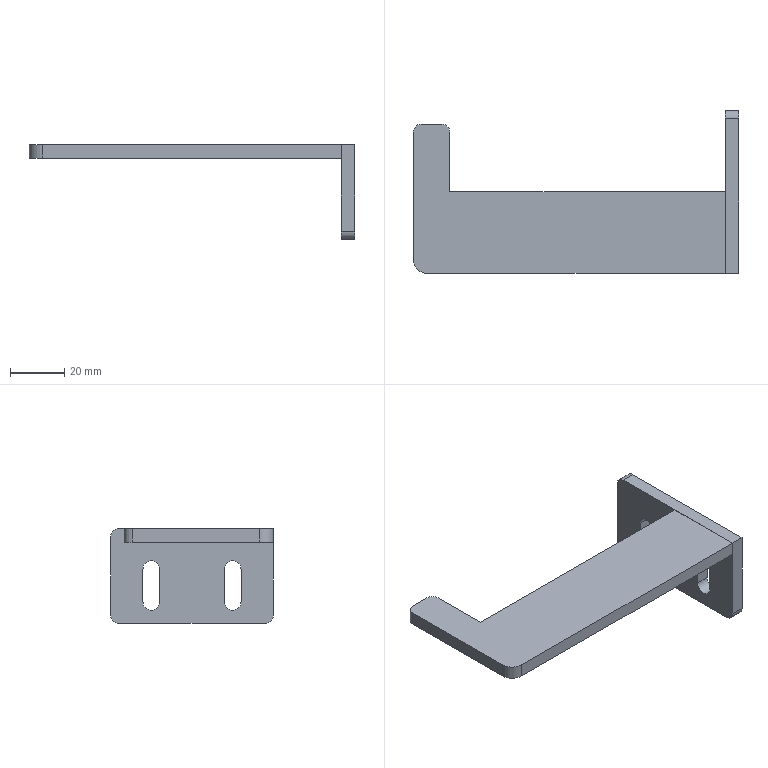Part | NX | features BREP 2 | 2 solids | 28 faces | box 120 x 60 x 35 mm | volume 28316 mm3 | plane 18 | cylinder 10 | commonest cylinder face diameters 6 x5 6.2 x4 10 x1
STEP:
#1=CARTESIAN_POINT('',(120.,33.1,-10.));
#2=VERTEX_POINT('',#1);
#3=CARTESIAN_POINT('',(120.,26.9,-10.));
#4=VERTEX_POINT('',#3);
#5=CARTESIAN_POINT('',(120.,30.,-10.));
#6=DIRECTION('',(1.,0.,0.));
#7=DIRECTION('',(0.,1.,0.));
#8=AXIS2_PLACEMENT_3D('',#5,#6,#7);
#9=CIRCLE('',#8,3.1);
#10=EDGE_CURVE('',#2,#4,#9,.T.);
#11=ORIENTED_EDGE('',*,*,#10,.T.);
#12=CARTESIAN_POINT('',(115.,26.9,-10.));
#13=VERTEX_POINT('',#12);
#14=CARTESIAN_POINT('',(145.,26.9,-10.));
#15=DIRECTION('',(-1.,0.,0.));
#16=VECTOR('',#15,1000.);
#17=LINE('',#14,#16);
#18=EDGE_CURVE('',#4,#13,#17,.T.);
#19=ORIENTED_EDGE('',*,*,#18,.T.);
#20=CARTESIAN_POINT('',(115.,33.1,-10.));
#21=VERTEX_POINT('',#20);
#22=CARTESIAN_POINT('',(115.,30.,-10.));
#23=DIRECTION('',(-1.,0.,0.));
#24=DIRECTION('',(0.,0.,1.));
#25=AXIS2_PLACEMENT_3D('',#22,#23,#24);
#26=CIRCLE('',#25,3.1);
#27=EDGE_CURVE('',#13,#21,#26,.T.);
#28=ORIENTED_EDGE('',*,*,#27,.T.);
#29=CARTESIAN_POINT('',(145.,33.1,-10.));
#30=DIRECTION('',(-1.,0.,0.));
#31=VECTOR('',#30,1000.);
#32=LINE('',#29,#31);
#33=EDGE_CURVE('',#2,#21,#32,.T.);
#34=ORIENTED_EDGE('',*,*,#33,.F.);
#35=EDGE_LOOP('',(#11,#19,#28,#34));
#36=FACE_BOUND('',#35,.T.);
#37=CARTESIAN_POINT('',(145.,30.,-10.));
#38=DIRECTION('',(-1.,0.,0.));
#39=DIRECTION('',(0.,0.,1.));
#40=AXIS2_PLACEMENT_3D('',#37,#38,#39);
#41=CYLINDRICAL_SURFACE('',#40,3.1);
#42=ADVANCED_FACE('',(#36),#41,.F.);
#43=CARTESIAN_POINT('',(120.,3.1,-10.));
#44=VERTEX_POINT('',#43);
#45=CARTESIAN_POINT('',(120.,-3.1,-10.));
#46=VERTEX_POINT('',#45);
#47=CARTESIAN_POINT('',(120.,0.,-10.));
#48=DIRECTION('',(1.,0.,0.));
#49=DIRECTION('',(0.,1.,0.));
#50=AXIS2_PLACEMENT_3D('',#47,#48,#49);
#51=CIRCLE('',#50,3.1);
#52=EDGE_CURVE('',#44,#46,#51,.T.);
#53=ORIENTED_EDGE('',*,*,#52,.T.);
#54=CARTESIAN_POINT('',(115.,-3.1,-10.));
#55=VERTEX_POINT('',#54);
#56=CARTESIAN_POINT('',(145.,-3.1,-10.));
#57=DIRECTION('',(-1.,0.,0.));
#58=VECTOR('',#57,1000.);
#59=LINE('',#56,#58);
#60=EDGE_CURVE('',#46,#55,#59,.T.);
#61=ORIENTED_EDGE('',*,*,#60,.T.);
#62=CARTESIAN_POINT('',(115.,3.1,-10.));
#63=VERTEX_POINT('',#62);
#64=CARTESIAN_POINT('',(115.,0.,-10.));
#65=DIRECTION('',(-1.,0.,0.));
#66=DIRECTION('',(0.,0.,-1.));
#67=AXIS2_PLACEMENT_3D('',#64,#65,#66);
#68=CIRCLE('',#67,3.1);
#69=EDGE_CURVE('',#55,#63,#68,.T.);
#70=ORIENTED_EDGE('',*,*,#69,.T.);
#71=CARTESIAN_POINT('',(145.,3.1,-10.));
#72=DIRECTION('',(-1.,0.,0.));
#73=VECTOR('',#72,1000.);
#74=LINE('',#71,#73);
#75=EDGE_CURVE('',#44,#63,#74,.T.);
#76=ORIENTED_EDGE('',*,*,#75,.F.);
#77=EDGE_LOOP('',(#53,#61,#70,#76));
#78=FACE_BOUND('',#77,.T.);
#79=CARTESIAN_POINT('',(145.,0.,-10.));
#80=DIRECTION('',(-1.,0.,0.));
#81=DIRECTION('',(0.,0.,1.));
#82=AXIS2_PLACEMENT_3D('',#79,#80,#81);
#83=CYLINDRICAL_SURFACE('',#82,3.1);
#84=ADVANCED_FACE('',(#78),#83,.F.);
#85=CARTESIAN_POINT('',(115.,33.1,-22.));
#86=VERTEX_POINT('',#85);
#87=CARTESIAN_POINT('',(115.,26.9,-22.));
#88=VERTEX_POINT('',#87);
#89=CARTESIAN_POINT('',(115.,30.,-22.));
#90=DIRECTION('',(-1.,0.,0.));
#91=DIRECTION('',(0.,0.,1.));
#92=AXIS2_PLACEMENT_3D('',#89,#90,#91);
#93=CIRCLE('',#92,3.1);
#94=EDGE_CURVE('',#86,#88,#93,.T.);
#95=ORIENTED_EDGE('',*,*,#94,.F.);
#96=CARTESIAN_POINT('',(115.,33.1,-22.));
#97=DIRECTION('',(0.,0.,-1.));
#98=VECTOR('',#97,1000.);
#99=LINE('',#96,#98);
#100=EDGE_CURVE('',#21,#86,#99,.T.);
#101=ORIENTED_EDGE('',*,*,#100,.F.);
#102=ORIENTED_EDGE('',*,*,#27,.F.);
#103=CARTESIAN_POINT('',(115.,26.9,-22.));
#104=DIRECTION('',(0.,0.,1.));
#105=VECTOR('',#104,1000.);
#106=LINE('',#103,#105);
#107=EDGE_CURVE('',#88,#13,#106,.T.);
#108=ORIENTED_EDGE('',*,*,#107,.F.);
#109=EDGE_LOOP('',(#95,#101,#102,#108));
#110=FACE_BOUND('',#109,.T.);
#111=ORIENTED_EDGE('',*,*,#69,.F.);
#112=CARTESIAN_POINT('',(115.,-3.1,-22.));
#113=VERTEX_POINT('',#112);
#114=CARTESIAN_POINT('',(115.,-3.1,-22.));
#115=DIRECTION('',(0.,0.,1.));
#116=VECTOR('',#115,1000.);
#117=LINE('',#114,#116);
#118=EDGE_CURVE('',#113,#55,#117,.T.);
#119=ORIENTED_EDGE('',*,*,#118,.F.);
#120=CARTESIAN_POINT('',(115.,3.1,-22.));
#121=VERTEX_POINT('',#120);
#122=CARTESIAN_POINT('',(115.,0.,-22.));
#123=DIRECTION('',(-1.,0.,0.));
#124=DIRECTION('',(0.,0.,-1.));
#125=AXIS2_PLACEMENT_3D('',#122,#123,#124);
#126=CIRCLE('',#125,3.1);
#127=EDGE_CURVE('',#121,#113,#126,.T.);
#128=ORIENTED_EDGE('',*,*,#127,.F.);
#129=CARTESIAN_POINT('',(115.,3.1,-22.));
#130=DIRECTION('',(0.,0.,-1.));
#131=VECTOR('',#130,1000.);
#132=LINE('',#129,#131);
#133=EDGE_CURVE('',#63,#121,#132,.T.);
#134=ORIENTED_EDGE('',*,*,#133,.F.);
#135=EDGE_LOOP('',(#111,#119,#128,#134));
#136=FACE_BOUND('',#135,.T.);
#137=CARTESIAN_POINT('',(115.,42.,5.));
#138=VERTEX_POINT('',#137);
#139=CARTESIAN_POINT('',(115.,-15.,5.));
#140=VERTEX_POINT('',#139);
#141=CARTESIAN_POINT('',(115.,45.,5.));
#142=DIRECTION('',(0.,-1.,0.));
#143=VECTOR('',#142,1000.);
#144=LINE('',#141,#143);
#145=EDGE_CURVE('',#138,#140,#144,.T.);
#146=ORIENTED_EDGE('',*,*,#145,.F.);
#147=CARTESIAN_POINT('',(115.,45.,2.));
#148=VERTEX_POINT('',#147);
#149=CARTESIAN_POINT('',(115.,42.,2.));
#150=DIRECTION('',(-1.,0.,0.));
#151=DIRECTION('',(0.,0.,1.));
#152=AXIS2_PLACEMENT_3D('',#149,#150,#151);
#153=CIRCLE('',#152,3.);
#154=EDGE_CURVE('',#138,#148,#153,.T.);
#155=ORIENTED_EDGE('',*,*,#154,.T.);
#156=CARTESIAN_POINT('',(115.,45.,-27.));
#157=VERTEX_POINT('',#156);
#158=CARTESIAN_POINT('',(115.,45.,-30.));
#159=DIRECTION('',(0.,0.,1.));
#160=VECTOR('',#159,1000.);
#161=LINE('',#158,#160);
#162=EDGE_CURVE('',#157,#148,#161,.T.);
#163=ORIENTED_EDGE('',*,*,#162,.F.);
#164=CARTESIAN_POINT('',(115.,42.,-30.));
#165=VERTEX_POINT('',#164);
#166=CARTESIAN_POINT('',(115.,42.,-27.));
#167=DIRECTION('',(-1.,0.,0.));
#168=DIRECTION('',(0.,0.,1.));
#169=AXIS2_PLACEMENT_3D('',#166,#167,#168);
#170=CIRCLE('',#169,3.);
#171=EDGE_CURVE('',#157,#165,#170,.T.);
#172=ORIENTED_EDGE('',*,*,#171,.T.);
#173=CARTESIAN_POINT('',(115.,-12.,-30.));
#174=VERTEX_POINT('',#173);
#175=CARTESIAN_POINT('',(115.,45.,-30.));
#176=DIRECTION('',(0.,-1.,0.));
#177=VECTOR('',#176,1000.);
#178=LINE('',#175,#177);
#179=EDGE_CURVE('',#165,#174,#178,.T.);
#180=ORIENTED_EDGE('',*,*,#179,.T.);
#181=CARTESIAN_POINT('',(115.,-15.,-27.));
#182=VERTEX_POINT('',#181);
#183=CARTESIAN_POINT('',(115.,-12.,-27.));
#184=DIRECTION('',(-1.,0.,0.));
#185=DIRECTION('',(0.,0.,1.));
#186=AXIS2_PLACEMENT_3D('',#183,#184,#185);
#187=CIRCLE('',#186,3.);
#188=EDGE_CURVE('',#174,#182,#187,.T.);
#189=ORIENTED_EDGE('',*,*,#188,.T.);
#190=CARTESIAN_POINT('',(115.,-15.,-30.));
#191=DIRECTION('',(0.,0.,1.));
#192=VECTOR('',#191,1000.);
#193=LINE('',#190,#192);
#194=EDGE_CURVE('',#182,#140,#193,.T.);
#195=ORIENTED_EDGE('',*,*,#194,.T.);
#196=EDGE_LOOP('',(#146,#155,#163,#172,#180,#189,#195));
#197=FACE_BOUND('',#196,.T.);
#198=CARTESIAN_POINT('',(115.,45.,-30.));
#199=DIRECTION('',(-1.,0.,0.));
#200=DIRECTION('',(0.,0.,1.));
#201=AXIS2_PLACEMENT_3D('',#198,#199,#200);
#202=PLANE('',#201);
#203=ADVANCED_FACE('',(#110,#136,#197),#202,.T.);
#204=ORIENTED_EDGE('',*,*,#162,.T.);
#205=CARTESIAN_POINT('',(120.,45.,2.));
#206=VERTEX_POINT('',#205);
#207=CARTESIAN_POINT('',(115.,45.,2.));
#208=DIRECTION('',(1.,0.,0.));
#209=VECTOR('',#208,1000.);
#210=LINE('',#207,#209);
#211=EDGE_CURVE('',#148,#206,#210,.T.);
#212=ORIENTED_EDGE('',*,*,#211,.T.);
#213=CARTESIAN_POINT('',(120.,45.,-27.));
#214=VERTEX_POINT('',#213);
#215=CARTESIAN_POINT('',(120.,45.,-30.));
#216=DIRECTION('',(0.,0.,1.));
#217=VECTOR('',#216,1000.);
#218=LINE('',#215,#217);
#219=EDGE_CURVE('',#214,#206,#218,.T.);
#220=ORIENTED_EDGE('',*,*,#219,.F.);
#221=CARTESIAN_POINT('',(115.,45.,-27.));
#222=DIRECTION('',(-1.,0.,0.));
#223=VECTOR('',#222,1000.);
#224=LINE('',#221,#223);
#225=EDGE_CURVE('',#214,#157,#224,.T.);
#226=ORIENTED_EDGE('',*,*,#225,.T.);
#227=EDGE_LOOP('',(#204,#212,#220,#226));
#228=FACE_BOUND('',#227,.T.);
#229=CARTESIAN_POINT('',(115.,45.,-30.));
#230=DIRECTION('',(0.,1.,0.));
#231=DIRECTION('',(0.,0.,1.));
#232=AXIS2_PLACEMENT_3D('',#229,#230,#231);
#233=PLANE('',#232);
#234=ADVANCED_FACE('',(#228),#233,.T.);
#235=CARTESIAN_POINT('',(120.,26.9,-22.));
#236=VERTEX_POINT('',#235);
#237=CARTESIAN_POINT('',(120.,33.1,-22.));
#238=VERTEX_POINT('',#237);
#239=CARTESIAN_POINT('',(120.,30.,-22.));
#240=DIRECTION('',(1.,0.,0.));
#241=DIRECTION('',(0.,1.,0.));
#242=AXIS2_PLACEMENT_3D('',#239,#240,#241);
#243=CIRCLE('',#242,3.1);
#244=EDGE_CURVE('',#236,#238,#243,.T.);
#245=ORIENTED_EDGE('',*,*,#244,.F.);
#246=CARTESIAN_POINT('',(120.,26.9,-30.));
#247=DIRECTION('',(0.,0.,-1.));
#248=VECTOR('',#247,1000.);
#249=LINE('',#246,#248);
#250=EDGE_CURVE('',#4,#236,#249,.T.);
#251=ORIENTED_EDGE('',*,*,#250,.F.);
#252=ORIENTED_EDGE('',*,*,#10,.F.);
#253=CARTESIAN_POINT('',(120.,33.1,-30.));
#254=DIRECTION('',(0.,0.,1.));
#255=VECTOR('',#254,1000.);
#256=LINE('',#253,#255);
#257=EDGE_CURVE('',#238,#2,#256,.T.);
#258=ORIENTED_EDGE('',*,*,#257,.F.);
#259=EDGE_LOOP('',(#245,#251,#252,#258));
#260=FACE_BOUND('',#259,.T.);
#261=ORIENTED_EDGE('',*,*,#52,.F.);
#262=CARTESIAN_POINT('',(120.,3.1,-22.));
#263=VERTEX_POINT('',#262);
#264=CARTESIAN_POINT('',(120.,3.1,-30.));
#265=DIRECTION('',(0.,0.,1.));
#266=VECTOR('',#265,1000.);
#267=LINE('',#264,#266);
#268=EDGE_CURVE('',#263,#44,#267,.T.);
#269=ORIENTED_EDGE('',*,*,#268,.F.);
#270=CARTESIAN_POINT('',(120.,-3.1,-22.));
#271=VERTEX_POINT('',#270);
#272=CARTESIAN_POINT('',(120.,0.,-22.));
#273=DIRECTION('',(1.,0.,0.));
#274=DIRECTION('',(0.,1.,0.));
#275=AXIS2_PLACEMENT_3D('',#272,#273,#274);
#276=CIRCLE('',#275,3.1);
#277=EDGE_CURVE('',#271,#263,#276,.T.);
#278=ORIENTED_EDGE('',*,*,#277,.F.);
#279=CARTESIAN_POINT('',(120.,-3.1,-30.));
#280=DIRECTION('',(0.,0.,-1.));
#281=VECTOR('',#280,1000.);
#282=LINE('',#279,#281);
#283=EDGE_CURVE('',#46,#271,#282,.T.);
#284=ORIENTED_EDGE('',*,*,#283,.F.);
#285=EDGE_LOOP('',(#261,#269,#278,#284));
#286=FACE_BOUND('',#285,.T.);
#287=ORIENTED_EDGE('',*,*,#219,.T.);
#288=CARTESIAN_POINT('',(120.,42.,5.));
#289=VERTEX_POINT('',#288);
#290=CARTESIAN_POINT('',(120.,42.,2.));
#291=DIRECTION('',(1.,0.,0.));
#292=DIRECTION('',(0.,1.,0.));
#293=AXIS2_PLACEMENT_3D('',#290,#291,#292);
#294=CIRCLE('',#293,3.);
#295=EDGE_CURVE('',#206,#289,#294,.T.);
#296=ORIENTED_EDGE('',*,*,#295,.T.);
#297=CARTESIAN_POINT('',(120.,-15.,5.));
#298=VERTEX_POINT('',#297);
#299=CARTESIAN_POINT('',(120.,45.,5.));
#300=DIRECTION('',(0.,1.,0.));
#301=VECTOR('',#300,1000.);
#302=LINE('',#299,#301);
#303=EDGE_CURVE('',#298,#289,#302,.T.);
#304=ORIENTED_EDGE('',*,*,#303,.F.);
#305=CARTESIAN_POINT('',(120.,-15.,-27.));
#306=VERTEX_POINT('',#305);
#307=CARTESIAN_POINT('',(120.,-15.,-30.));
#308=DIRECTION('',(0.,0.,1.));
#309=VECTOR('',#308,1000.);
#310=LINE('',#307,#309);
#311=EDGE_CURVE('',#306,#298,#310,.T.);
#312=ORIENTED_EDGE('',*,*,#311,.F.);
#313=CARTESIAN_POINT('',(120.,-12.,-30.));
#314=VERTEX_POINT('',#313);
#315=CARTESIAN_POINT('',(120.,-12.,-27.));
#316=DIRECTION('',(1.,0.,0.));
#317=DIRECTION('',(0.,1.,0.));
#318=AXIS2_PLACEMENT_3D('',#315,#316,#317);
#319=CIRCLE('',#318,3.);
#320=EDGE_CURVE('',#306,#314,#319,.T.);
#321=ORIENTED_EDGE('',*,*,#320,.T.);
#322=CARTESIAN_POINT('',(120.,42.,-30.));
#323=VERTEX_POINT('',#322);
#324=CARTESIAN_POINT('',(120.,45.,-30.));
#325=DIRECTION('',(0.,1.,0.));
#326=VECTOR('',#325,1000.);
#327=LINE('',#324,#326);
#328=EDGE_CURVE('',#314,#323,#327,.T.);
#329=ORIENTED_EDGE('',*,*,#328,.T.);
#330=CARTESIAN_POINT('',(120.,42.,-27.));
#331=DIRECTION('',(1.,0.,0.));
#332=DIRECTION('',(0.,1.,0.));
#333=AXIS2_PLACEMENT_3D('',#330,#331,#332);
#334=CIRCLE('',#333,3.);
#335=EDGE_CURVE('',#323,#214,#334,.T.);
#336=ORIENTED_EDGE('',*,*,#335,.T.);
#337=EDGE_LOOP('',(#287,#296,#304,#312,#321,#329,#336));
#338=FACE_BOUND('',#337,.T.);
#339=CARTESIAN_POINT('',(120.,45.,-30.));
#340=DIRECTION('',(1.,0.,0.));
#341=DIRECTION('',(0.,1.,0.));
#342=AXIS2_PLACEMENT_3D('',#339,#340,#341);
#343=PLANE('',#342);
#344=ADVANCED_FACE('',(#260,#286,#338),#343,.T.);
#345=ORIENTED_EDGE('',*,*,#194,.F.);
#346=CARTESIAN_POINT('',(120.,-15.,-27.));
#347=DIRECTION('',(1.,0.,0.));
#348=VECTOR('',#347,1000.);
#349=LINE('',#346,#348);
#350=EDGE_CURVE('',#182,#306,#349,.T.);
#351=ORIENTED_EDGE('',*,*,#350,.T.);
#352=ORIENTED_EDGE('',*,*,#311,.T.);
#353=CARTESIAN_POINT('',(115.,-15.,5.));
#354=DIRECTION('',(1.,0.,0.));
#355=VECTOR('',#354,1000.);
#356=LINE('',#353,#355);
#357=EDGE_CURVE('',#140,#298,#356,.T.);
#358=ORIENTED_EDGE('',*,*,#357,.F.);
#359=EDGE_LOOP('',(#345,#351,#352,#358));
#360=FACE_BOUND('',#359,.T.);
#361=CARTESIAN_POINT('',(115.,-15.,-30.));
#362=DIRECTION('',(0.,-1.,0.));
#363=DIRECTION('',(0.,0.,-1.));
#364=AXIS2_PLACEMENT_3D('',#361,#362,#363);
#365=PLANE('',#364);
#366=ADVANCED_FACE('',(#360),#365,.T.);
#367=ORIENTED_EDGE('',*,*,#328,.F.);
#368=CARTESIAN_POINT('',(115.,-12.,-30.));
#369=DIRECTION('',(-1.,0.,0.));
#370=VECTOR('',#369,1000.);
#371=LINE('',#368,#370);
#372=EDGE_CURVE('',#314,#174,#371,.T.);
#373=ORIENTED_EDGE('',*,*,#372,.T.);
#374=ORIENTED_EDGE('',*,*,#179,.F.);
#375=CARTESIAN_POINT('',(120.,42.,-30.));
#376=DIRECTION('',(1.,0.,0.));
#377=VECTOR('',#376,1000.);
#378=LINE('',#375,#377);
#379=EDGE_CURVE('',#165,#323,#378,.T.);
#380=ORIENTED_EDGE('',*,*,#379,.T.);
#381=EDGE_LOOP('',(#367,#373,#374,#380));
#382=FACE_BOUND('',#381,.T.);
#383=CARTESIAN_POINT('',(0.,0.,-30.));
#384=DIRECTION('',(0.,0.,1.));
#385=DIRECTION('',(1.,0.,0.));
#386=AXIS2_PLACEMENT_3D('',#383,#384,#385);
#387=PLANE('',#386);
#388=ADVANCED_FACE('',(#382),#387,.F.);
#389=ORIENTED_EDGE('',*,*,#303,.T.);
#390=CARTESIAN_POINT('',(0.,42.,5.));
#391=DIRECTION('',(-1.,0.,0.));
#392=VECTOR('',#391,1000.);
#393=LINE('',#390,#392);
#394=EDGE_CURVE('',#289,#138,#393,.T.);
#395=ORIENTED_EDGE('',*,*,#394,.T.);
#396=ORIENTED_EDGE('',*,*,#145,.T.);
#397=ORIENTED_EDGE('',*,*,#357,.T.);
#398=EDGE_LOOP('',(#389,#395,#396,#397));
#399=FACE_BOUND('',#398,.T.);
#400=CARTESIAN_POINT('',(0.,0.,5.));
#401=DIRECTION('',(0.,0.,1.));
#402=DIRECTION('',(1.,0.,0.));
#403=AXIS2_PLACEMENT_3D('',#400,#401,#402);
#404=PLANE('',#403);
#405=ADVANCED_FACE('',(#399),#404,.T.);
#406=ORIENTED_EDGE('',*,*,#188,.F.);
#407=ORIENTED_EDGE('',*,*,#372,.F.);
#408=ORIENTED_EDGE('',*,*,#320,.F.);
#409=ORIENTED_EDGE('',*,*,#350,.F.);
#410=EDGE_LOOP('',(#406,#407,#408,#409));
#411=FACE_BOUND('',#410,.T.);
#412=CARTESIAN_POINT('',(115.,-12.,-27.));
#413=DIRECTION('',(-1.,0.,0.));
#414=DIRECTION('',(0.,0.,1.));
#415=AXIS2_PLACEMENT_3D('',#412,#413,#414);
#416=CYLINDRICAL_SURFACE('',#415,3.);
#417=ADVANCED_FACE('',(#411),#416,.T.);
#418=ORIENTED_EDGE('',*,*,#335,.F.);
#419=ORIENTED_EDGE('',*,*,#379,.F.);
#420=ORIENTED_EDGE('',*,*,#171,.F.);
#421=ORIENTED_EDGE('',*,*,#225,.F.);
#422=EDGE_LOOP('',(#418,#419,#420,#421));
#423=FACE_BOUND('',#422,.T.);
#424=CARTESIAN_POINT('',(115.,42.,-27.));
#425=DIRECTION('',(1.,0.,0.));
#426=DIRECTION('',(0.,0.,-1.));
#427=AXIS2_PLACEMENT_3D('',#424,#425,#426);
#428=CYLINDRICAL_SURFACE('',#427,3.);
#429=ADVANCED_FACE('',(#423),#428,.T.);
#430=ORIENTED_EDGE('',*,*,#283,.T.);
#431=CARTESIAN_POINT('',(145.,-3.1,-22.));
#432=DIRECTION('',(-1.,0.,0.));
#433=VECTOR('',#432,1000.);
#434=LINE('',#431,#433);
#435=EDGE_CURVE('',#271,#113,#434,.T.);
#436=ORIENTED_EDGE('',*,*,#435,.T.);
#437=ORIENTED_EDGE('',*,*,#118,.T.);
#438=ORIENTED_EDGE('',*,*,#60,.F.);
#439=EDGE_LOOP('',(#430,#436,#437,#438));
#440=FACE_BOUND('',#439,.T.);
#441=CARTESIAN_POINT('',(145.,-3.1,-22.));
#442=DIRECTION('',(0.,-1.,0.));
#443=DIRECTION('',(0.,0.,-1.));
#444=AXIS2_PLACEMENT_3D('',#441,#442,#443);
#445=PLANE('',#444);
#446=ADVANCED_FACE('',(#440),#445,.F.);
#447=ORIENTED_EDGE('',*,*,#277,.T.);
#448=CARTESIAN_POINT('',(145.,3.1,-22.));
#449=DIRECTION('',(-1.,0.,0.));
#450=VECTOR('',#449,1000.);
#451=LINE('',#448,#450);
#452=EDGE_CURVE('',#263,#121,#451,.T.);
#453=ORIENTED_EDGE('',*,*,#452,.T.);
#454=ORIENTED_EDGE('',*,*,#127,.T.);
#455=ORIENTED_EDGE('',*,*,#435,.F.);
#456=EDGE_LOOP('',(#447,#453,#454,#455));
#457=FACE_BOUND('',#456,.T.);
#458=CARTESIAN_POINT('',(145.,0.,-22.));
#459=DIRECTION('',(-1.,0.,0.));
#460=DIRECTION('',(0.,0.,1.));
#461=AXIS2_PLACEMENT_3D('',#458,#459,#460);
#462=CYLINDRICAL_SURFACE('',#461,3.1);
#463=ADVANCED_FACE('',(#457),#462,.F.);
#464=ORIENTED_EDGE('',*,*,#268,.T.);
#465=ORIENTED_EDGE('',*,*,#75,.T.);
#466=ORIENTED_EDGE('',*,*,#133,.T.);
#467=ORIENTED_EDGE('',*,*,#452,.F.);
#468=EDGE_LOOP('',(#464,#465,#466,#467));
#469=FACE_BOUND('',#468,.T.);
#470=CARTESIAN_POINT('',(145.,3.1,-22.));
#471=DIRECTION('',(0.,1.,0.));
#472=DIRECTION('',(0.,0.,1.));
#473=AXIS2_PLACEMENT_3D('',#470,#471,#472);
#474=PLANE('',#473);
#475=ADVANCED_FACE('',(#469),#474,.F.);
#476=ORIENTED_EDGE('',*,*,#244,.T.);
#477=CARTESIAN_POINT('',(145.,33.1,-22.));
#478=DIRECTION('',(-1.,0.,0.));
#479=VECTOR('',#478,1000.);
#480=LINE('',#477,#479);
#481=EDGE_CURVE('',#238,#86,#480,.T.);
#482=ORIENTED_EDGE('',*,*,#481,.T.);
#483=ORIENTED_EDGE('',*,*,#94,.T.);
#484=CARTESIAN_POINT('',(145.,26.9,-22.));
#485=DIRECTION('',(-1.,0.,0.));
#486=VECTOR('',#485,1000.);
#487=LINE('',#484,#486);
#488=EDGE_CURVE('',#236,#88,#487,.T.);
#489=ORIENTED_EDGE('',*,*,#488,.F.);
#490=EDGE_LOOP('',(#476,#482,#483,#489));
#491=FACE_BOUND('',#490,.T.);
#492=CARTESIAN_POINT('',(145.,30.,-22.));
#493=DIRECTION('',(-1.,0.,0.));
#494=DIRECTION('',(0.,0.,1.));
#495=AXIS2_PLACEMENT_3D('',#492,#493,#494);
#496=CYLINDRICAL_SURFACE('',#495,3.1);
#497=ADVANCED_FACE('',(#491),#496,.F.);
#498=ORIENTED_EDGE('',*,*,#257,.T.);
#499=ORIENTED_EDGE('',*,*,#33,.T.);
#500=ORIENTED_EDGE('',*,*,#100,.T.);
#501=ORIENTED_EDGE('',*,*,#481,.F.);
#502=EDGE_LOOP('',(#498,#499,#500,#501));
#503=FACE_BOUND('',#502,.T.);
#504=CARTESIAN_POINT('',(145.,33.1,-22.));
#505=DIRECTION('',(0.,1.,0.));
#506=DIRECTION('',(0.,0.,1.));
#507=AXIS2_PLACEMENT_3D('',#504,#505,#506);
#508=PLANE('',#507);
#509=ADVANCED_FACE('',(#503),#508,.F.);
#510=ORIENTED_EDGE('',*,*,#250,.T.);
#511=ORIENTED_EDGE('',*,*,#488,.T.);
#512=ORIENTED_EDGE('',*,*,#107,.T.);
#513=ORIENTED_EDGE('',*,*,#18,.F.);
#514=EDGE_LOOP('',(#510,#511,#512,#513));
#515=FACE_BOUND('',#514,.T.);
#516=CARTESIAN_POINT('',(145.,26.9,-22.));
#517=DIRECTION('',(0.,-1.,0.));
#518=DIRECTION('',(0.,0.,-1.));
#519=AXIS2_PLACEMENT_3D('',#516,#517,#518);
#520=PLANE('',#519);
#521=ADVANCED_FACE('',(#515),#520,.F.);
#522=ORIENTED_EDGE('',*,*,#295,.F.);
#523=ORIENTED_EDGE('',*,*,#211,.F.);
#524=ORIENTED_EDGE('',*,*,#154,.F.);
#525=ORIENTED_EDGE('',*,*,#394,.F.);
#526=EDGE_LOOP('',(#522,#523,#524,#525));
#527=FACE_BOUND('',#526,.T.);
#528=CARTESIAN_POINT('',(0.,42.,2.));
#529=DIRECTION('',(-1.,0.,0.));
#530=DIRECTION('',(0.,0.,1.));
#531=AXIS2_PLACEMENT_3D('',#528,#529,#530);
#532=CYLINDRICAL_SURFACE('',#531,3.);
#533=ADVANCED_FACE('',(#527),#532,.T.);
#534=CLOSED_SHELL('',(#42,#84,#203,#234,#344,#366,#388,#405,#417,#429,#446,#463,#475,#497,#509,#521,#533));
#535=MANIFOLD_SOLID_BREP('',#534);
#536=CARTESIAN_POINT('',(5.,-15.,5.));
#537=VERTEX_POINT('',#536);
#538=CARTESIAN_POINT('',(115.,-15.,5.));
#539=VERTEX_POINT('',#538);
#540=CARTESIAN_POINT('',(0.,-15.,5.));
#541=DIRECTION('',(1.,0.,0.));
#542=VECTOR('',#541,1000.);
#543=LINE('',#540,#542);
#544=EDGE_CURVE('',#537,#539,#543,.T.);
#545=ORIENTED_EDGE('',*,*,#544,.F.);
#546=CARTESIAN_POINT('',(5.,-15.,0.));
#547=VERTEX_POINT('',#546);
#548=CARTESIAN_POINT('',(5.,-15.,5.));
#549=DIRECTION('',(0.,0.,-1.));
#550=VECTOR('',#549,1000.);
#551=LINE('',#548,#550);
#552=EDGE_CURVE('',#537,#547,#551,.T.);
#553=ORIENTED_EDGE('',*,*,#552,.T.);
#554=CARTESIAN_POINT('',(115.,-15.,0.));
#555=VERTEX_POINT('',#554);
#556=CARTESIAN_POINT('',(0.,-15.,0.));
#557=DIRECTION('',(1.,0.,0.));
#558=VECTOR('',#557,1000.);
#559=LINE('',#556,#558);
#560=EDGE_CURVE('',#547,#555,#559,.T.);
#561=ORIENTED_EDGE('',*,*,#560,.T.);
#562=CARTESIAN_POINT('',(115.,-15.,5.));
#563=DIRECTION('',(0.,0.,-1.));
#564=VECTOR('',#563,1000.);
#565=LINE('',#562,#564);
#566=EDGE_CURVE('',#539,#555,#565,.T.);
#567=ORIENTED_EDGE('',*,*,#566,.F.);
#568=EDGE_LOOP('',(#545,#553,#561,#567));
#569=FACE_BOUND('',#568,.T.);
#570=CARTESIAN_POINT('',(0.,-15.,5.));
#571=DIRECTION('',(0.,1.,0.));
#572=DIRECTION('',(0.,0.,1.));
#573=AXIS2_PLACEMENT_3D('',#570,#571,#572);
#574=PLANE('',#573);
#575=ADVANCED_FACE('',(#569),#574,.F.);
#576=CARTESIAN_POINT('',(115.,15.,0.));
#577=VERTEX_POINT('',#576);
#578=CARTESIAN_POINT('',(115.,15.,0.));
#579=DIRECTION('',(0.,1.,0.));
#580=VECTOR('',#579,1000.);
#581=LINE('',#578,#580);
#582=EDGE_CURVE('',#555,#577,#581,.T.);
#583=ORIENTED_EDGE('',*,*,#582,.T.);
#584=CARTESIAN_POINT('',(115.,15.,5.));
#585=VERTEX_POINT('',#584);
#586=CARTESIAN_POINT('',(115.,15.,5.));
#587=DIRECTION('',(0.,0.,-1.));
#588=VECTOR('',#587,1000.);
#589=LINE('',#586,#588);
#590=EDGE_CURVE('',#585,#577,#589,.T.);
#591=ORIENTED_EDGE('',*,*,#590,.F.);
#592=CARTESIAN_POINT('',(115.,15.,5.));
#593=DIRECTION('',(0.,1.,0.));
#594=VECTOR('',#593,1000.);
#595=LINE('',#592,#594);
#596=EDGE_CURVE('',#539,#585,#595,.T.);
#597=ORIENTED_EDGE('',*,*,#596,.F.);
#598=ORIENTED_EDGE('',*,*,#566,.T.);
#599=EDGE_LOOP('',(#583,#591,#597,#598));
#600=FACE_BOUND('',#599,.T.);
#601=CARTESIAN_POINT('',(115.,15.,5.));
#602=DIRECTION('',(-1.,0.,0.));
#603=DIRECTION('',(0.,0.,1.));
#604=AXIS2_PLACEMENT_3D('',#601,#602,#603);
#605=PLANE('',#604);
#606=ADVANCED_FACE('',(#600),#605,.F.);
#607=CARTESIAN_POINT('',(13.5,15.,0.));
#608=VERTEX_POINT('',#607);
#609=CARTESIAN_POINT('',(13.5,15.,0.));
#610=DIRECTION('',(-1.,0.,0.));
#611=VECTOR('',#610,1000.);
#612=LINE('',#609,#611);
#613=EDGE_CURVE('',#577,#608,#612,.T.);
#614=ORIENTED_EDGE('',*,*,#613,.T.);
#615=CARTESIAN_POINT('',(13.5,15.,5.));
#616=VERTEX_POINT('',#615);
#617=CARTESIAN_POINT('',(13.5,15.,5.));
#618=DIRECTION('',(0.,0.,-1.));
#619=VECTOR('',#618,1000.);
#620=LINE('',#617,#619);
#621=EDGE_CURVE('',#616,#608,#620,.T.);
#622=ORIENTED_EDGE('',*,*,#621,.F.);
#623=CARTESIAN_POINT('',(13.5,15.,5.));
#624=DIRECTION('',(-1.,0.,0.));
#625=VECTOR('',#624,1000.);
#626=LINE('',#623,#625);
#627=EDGE_CURVE('',#585,#616,#626,.T.);
#628=ORIENTED_EDGE('',*,*,#627,.F.);
#629=ORIENTED_EDGE('',*,*,#590,.T.);
#630=EDGE_LOOP('',(#614,#622,#628,#629));
#631=FACE_BOUND('',#630,.T.);
#632=CARTESIAN_POINT('',(13.5,15.,5.));
#633=DIRECTION('',(0.,-1.,0.));
#634=DIRECTION('',(1.,0.,0.));
#635=AXIS2_PLACEMENT_3D('',#632,#633,#634);
#636=PLANE('',#635);
#637=ADVANCED_FACE('',(#631),#636,.F.);
#638=CARTESIAN_POINT('',(13.5,37.,0.));
#639=VERTEX_POINT('',#638);
#640=CARTESIAN_POINT('',(13.5,40.,0.));
#641=DIRECTION('',(0.,1.,0.));
#642=VECTOR('',#641,1000.);
#643=LINE('',#640,#642);
#644=EDGE_CURVE('',#608,#639,#643,.T.);
#645=ORIENTED_EDGE('',*,*,#644,.T.);
#646=CARTESIAN_POINT('',(13.5,37.,5.));
#647=VERTEX_POINT('',#646);
#648=CARTESIAN_POINT('',(13.5,37.,5.));
#649=DIRECTION('',(0.,0.,1.));
#650=VECTOR('',#649,1000.);
#651=LINE('',#648,#650);
#652=EDGE_CURVE('',#639,#647,#651,.T.);
#653=ORIENTED_EDGE('',*,*,#652,.T.);
#654=CARTESIAN_POINT('',(13.5,40.,5.));
#655=DIRECTION('',(0.,1.,0.));
#656=VECTOR('',#655,1000.);
#657=LINE('',#654,#656);
#658=EDGE_CURVE('',#616,#647,#657,.T.);
#659=ORIENTED_EDGE('',*,*,#658,.F.);
#660=ORIENTED_EDGE('',*,*,#621,.T.);
#661=EDGE_LOOP('',(#645,#653,#659,#660));
#662=FACE_BOUND('',#661,.T.);
#663=CARTESIAN_POINT('',(13.5,40.,5.));
#664=DIRECTION('',(-1.,0.,0.));
#665=DIRECTION('',(0.,-1.,0.));
#666=AXIS2_PLACEMENT_3D('',#663,#664,#665);
#667=PLANE('',#666);
#668=ADVANCED_FACE('',(#662),#667,.F.);
#669=CARTESIAN_POINT('',(10.5,40.,5.));
#670=VERTEX_POINT('',#669);
#671=CARTESIAN_POINT('',(3.,40.,5.));
#672=VERTEX_POINT('',#671);
#673=CARTESIAN_POINT('',(0.,40.,5.));
#674=DIRECTION('',(-1.,0.,0.));
#675=VECTOR('',#674,1000.);
#676=LINE('',#673,#675);
#677=EDGE_CURVE('',#670,#672,#676,.T.);
#678=ORIENTED_EDGE('',*,*,#677,.F.);
#679=CARTESIAN_POINT('',(10.5,40.,0.));
#680=VERTEX_POINT('',#679);
#681=CARTESIAN_POINT('',(10.5,40.,5.));
#682=DIRECTION('',(0.,0.,-1.));
#683=VECTOR('',#682,1000.);
#684=LINE('',#681,#683);
#685=EDGE_CURVE('',#670,#680,#684,.T.);
#686=ORIENTED_EDGE('',*,*,#685,.T.);
#687=CARTESIAN_POINT('',(3.,40.,0.));
#688=VERTEX_POINT('',#687);
#689=CARTESIAN_POINT('',(0.,40.,0.));
#690=DIRECTION('',(-1.,0.,0.));
#691=VECTOR('',#690,1000.);
#692=LINE('',#689,#691);
#693=EDGE_CURVE('',#680,#688,#692,.T.);
#694=ORIENTED_EDGE('',*,*,#693,.T.);
#695=CARTESIAN_POINT('',(3.,40.,5.));
#696=DIRECTION('',(0.,0.,1.));
#697=VECTOR('',#696,1000.);
#698=LINE('',#695,#697);
#699=EDGE_CURVE('',#688,#672,#698,.T.);
#700=ORIENTED_EDGE('',*,*,#699,.T.);
#701=EDGE_LOOP('',(#678,#686,#694,#700));
#702=FACE_BOUND('',#701,.T.);
#703=CARTESIAN_POINT('',(0.,40.,5.));
#704=DIRECTION('',(0.,-1.,0.));
#705=DIRECTION('',(0.,0.,-1.));
#706=AXIS2_PLACEMENT_3D('',#703,#704,#705);
#707=PLANE('',#706);
#708=ADVANCED_FACE('',(#702),#707,.F.);
#709=CARTESIAN_POINT('',(0.,37.,0.));
#710=VERTEX_POINT('',#709);
#711=CARTESIAN_POINT('',(0.,-10.,0.));
#712=VERTEX_POINT('',#711);
#713=CARTESIAN_POINT('',(0.,40.,0.));
#714=DIRECTION('',(0.,-1.,0.));
#715=VECTOR('',#714,1000.);
#716=LINE('',#713,#715);
#717=EDGE_CURVE('',#710,#712,#716,.T.);
#718=ORIENTED_EDGE('',*,*,#717,.T.);
#719=CARTESIAN_POINT('',(0.,-10.,5.));
#720=VERTEX_POINT('',#719);
#721=CARTESIAN_POINT('',(0.,-10.,5.));
#722=DIRECTION('',(0.,0.,1.));
#723=VECTOR('',#722,1000.);
#724=LINE('',#721,#723);
#725=EDGE_CURVE('',#712,#720,#724,.T.);
#726=ORIENTED_EDGE('',*,*,#725,.T.);
#727=CARTESIAN_POINT('',(0.,37.,5.));
#728=VERTEX_POINT('',#727);
#729=CARTESIAN_POINT('',(0.,40.,5.));
#730=DIRECTION('',(0.,-1.,0.));
#731=VECTOR('',#730,1000.);
#732=LINE('',#729,#731);
#733=EDGE_CURVE('',#728,#720,#732,.T.);
#734=ORIENTED_EDGE('',*,*,#733,.F.);
#735=CARTESIAN_POINT('',(0.,37.,5.));
#736=DIRECTION('',(0.,0.,-1.));
#737=VECTOR('',#736,1000.);
#738=LINE('',#735,#737);
#739=EDGE_CURVE('',#728,#710,#738,.T.);
#740=ORIENTED_EDGE('',*,*,#739,.T.);
#741=EDGE_LOOP('',(#718,#726,#734,#740));
#742=FACE_BOUND('',#741,.T.);
#743=CARTESIAN_POINT('',(0.,40.,5.));
#744=DIRECTION('',(1.,0.,0.));
#745=DIRECTION('',(0.,1.,0.));
#746=AXIS2_PLACEMENT_3D('',#743,#744,#745);
#747=PLANE('',#746);
#748=ADVANCED_FACE('',(#742),#747,.F.);
#749=ORIENTED_EDGE('',*,*,#733,.T.);
#750=CARTESIAN_POINT('',(5.,-10.,5.));
#751=DIRECTION('',(0.,0.,1.));
#752=DIRECTION('',(-1.,0.,0.));
#753=AXIS2_PLACEMENT_3D('',#750,#751,#752);
#754=CIRCLE('',#753,5.);
#755=EDGE_CURVE('',#720,#537,#754,.T.);
#756=ORIENTED_EDGE('',*,*,#755,.T.);
#757=ORIENTED_EDGE('',*,*,#544,.T.);
#758=ORIENTED_EDGE('',*,*,#596,.T.);
#759=ORIENTED_EDGE('',*,*,#627,.T.);
#760=ORIENTED_EDGE('',*,*,#658,.T.);
#761=CARTESIAN_POINT('',(10.5,37.,5.));
#762=DIRECTION('',(0.,0.,1.));
#763=DIRECTION('',(-1.,0.,0.));
#764=AXIS2_PLACEMENT_3D('',#761,#762,#763);
#765=CIRCLE('',#764,3.);
#766=EDGE_CURVE('',#647,#670,#765,.T.);
#767=ORIENTED_EDGE('',*,*,#766,.T.);
#768=ORIENTED_EDGE('',*,*,#677,.T.);
#769=CARTESIAN_POINT('',(3.,37.,5.));
#770=DIRECTION('',(0.,0.,1.));
#771=DIRECTION('',(-1.,0.,0.));
#772=AXIS2_PLACEMENT_3D('',#769,#770,#771);
#773=CIRCLE('',#772,3.);
#774=EDGE_CURVE('',#672,#728,#773,.T.);
#775=ORIENTED_EDGE('',*,*,#774,.T.);
#776=EDGE_LOOP('',(#749,#756,#757,#758,#759,#760,#767,#768,#775));
#777=FACE_BOUND('',#776,.T.);
#778=CARTESIAN_POINT('',(0.,0.,5.));
#779=DIRECTION('',(0.,0.,-1.));
#780=DIRECTION('',(-1.,0.,0.));
#781=AXIS2_PLACEMENT_3D('',#778,#779,#780);
#782=PLANE('',#781);
#783=ADVANCED_FACE('',(#777),#782,.F.);
#784=ORIENTED_EDGE('',*,*,#560,.F.);
#785=CARTESIAN_POINT('',(5.,-10.,0.));
#786=DIRECTION('',(0.,0.,-1.));
#787=DIRECTION('',(-1.,0.,0.));
#788=AXIS2_PLACEMENT_3D('',#785,#786,#787);
#789=CIRCLE('',#788,5.);
#790=EDGE_CURVE('',#547,#712,#789,.T.);
#791=ORIENTED_EDGE('',*,*,#790,.T.);
#792=ORIENTED_EDGE('',*,*,#717,.F.);
#793=CARTESIAN_POINT('',(3.,37.,0.));
#794=DIRECTION('',(0.,0.,-1.));
#795=DIRECTION('',(-1.,0.,0.));
#796=AXIS2_PLACEMENT_3D('',#793,#794,#795);
#797=CIRCLE('',#796,3.);
#798=EDGE_CURVE('',#710,#688,#797,.T.);
#799=ORIENTED_EDGE('',*,*,#798,.T.);
#800=ORIENTED_EDGE('',*,*,#693,.F.);
#801=CARTESIAN_POINT('',(10.5,37.,0.));
#802=DIRECTION('',(0.,0.,-1.));
#803=DIRECTION('',(-1.,0.,0.));
#804=AXIS2_PLACEMENT_3D('',#801,#802,#803);
#805=CIRCLE('',#804,3.);
#806=EDGE_CURVE('',#680,#639,#805,.T.);
#807=ORIENTED_EDGE('',*,*,#806,.T.);
#808=ORIENTED_EDGE('',*,*,#644,.F.);
#809=ORIENTED_EDGE('',*,*,#613,.F.);
#810=ORIENTED_EDGE('',*,*,#582,.F.);
#811=EDGE_LOOP('',(#784,#791,#792,#799,#800,#807,#808,#809,#810));
#812=FACE_BOUND('',#811,.T.);
#813=CARTESIAN_POINT('',(0.,0.,0.));
#814=DIRECTION('',(0.,0.,-1.));
#815=DIRECTION('',(-1.,0.,0.));
#816=AXIS2_PLACEMENT_3D('',#813,#814,#815);
#817=PLANE('',#816);
#818=ADVANCED_FACE('',(#812),#817,.T.);
#819=ORIENTED_EDGE('',*,*,#766,.F.);
#820=ORIENTED_EDGE('',*,*,#652,.F.);
#821=ORIENTED_EDGE('',*,*,#806,.F.);
#822=ORIENTED_EDGE('',*,*,#685,.F.);
#823=EDGE_LOOP('',(#819,#820,#821,#822));
#824=FACE_BOUND('',#823,.T.);
#825=CARTESIAN_POINT('',(10.5,37.,5.));
#826=DIRECTION('',(0.,0.,-1.));
#827=DIRECTION('',(-1.,0.,0.));
#828=AXIS2_PLACEMENT_3D('',#825,#826,#827);
#829=CYLINDRICAL_SURFACE('',#828,3.);
#830=ADVANCED_FACE('',(#824),#829,.T.);
#831=ORIENTED_EDGE('',*,*,#774,.F.);
#832=ORIENTED_EDGE('',*,*,#699,.F.);
#833=ORIENTED_EDGE('',*,*,#798,.F.);
#834=ORIENTED_EDGE('',*,*,#739,.F.);
#835=EDGE_LOOP('',(#831,#832,#833,#834));
#836=FACE_BOUND('',#835,.T.);
#837=CARTESIAN_POINT('',(3.,37.,5.));
#838=DIRECTION('',(0.,0.,-1.));
#839=DIRECTION('',(-1.,0.,0.));
#840=AXIS2_PLACEMENT_3D('',#837,#838,#839);
#841=CYLINDRICAL_SURFACE('',#840,3.);
#842=ADVANCED_FACE('',(#836),#841,.T.);
#843=ORIENTED_EDGE('',*,*,#755,.F.);
#844=ORIENTED_EDGE('',*,*,#725,.F.);
#845=ORIENTED_EDGE('',*,*,#790,.F.);
#846=ORIENTED_EDGE('',*,*,#552,.F.);
#847=EDGE_LOOP('',(#843,#844,#845,#846));
#848=FACE_BOUND('',#847,.T.);
#849=CARTESIAN_POINT('',(5.,-10.,5.));
#850=DIRECTION('',(0.,0.,-1.));
#851=DIRECTION('',(-1.,0.,0.));
#852=AXIS2_PLACEMENT_3D('',#849,#850,#851);
#853=CYLINDRICAL_SURFACE('',#852,5.);
#854=ADVANCED_FACE('',(#848),#853,.T.);
#855=CLOSED_SHELL('',(#575,#606,#637,#668,#708,#748,#783,#818,#830,#842,#854));
#856=MANIFOLD_SOLID_BREP('',#855);
#857=(LENGTH_UNIT()NAMED_UNIT(*)SI_UNIT(.MILLI.,.METRE.));
#858=UNCERTAINTY_MEASURE_WITH_UNIT(LENGTH_MEASURE(0.00001),#857,'','');
#859=(NAMED_UNIT(*)PLANE_ANGLE_UNIT()SI_UNIT($,.RADIAN.));
#860=(NAMED_UNIT(*)SI_UNIT($,.STERADIAN.)SOLID_ANGLE_UNIT());
#861=(GEOMETRIC_REPRESENTATION_CONTEXT(3)GLOBAL_UNCERTAINTY_ASSIGNED_CONTEXT((#858))GLOBAL_UNIT_ASSIGNED_CONTEXT((#857,#859,#860))REPRESENTATION_CONTEXT('',''));
#862=ADVANCED_BREP_SHAPE_REPRESENTATION('',(#535,#856),#861);